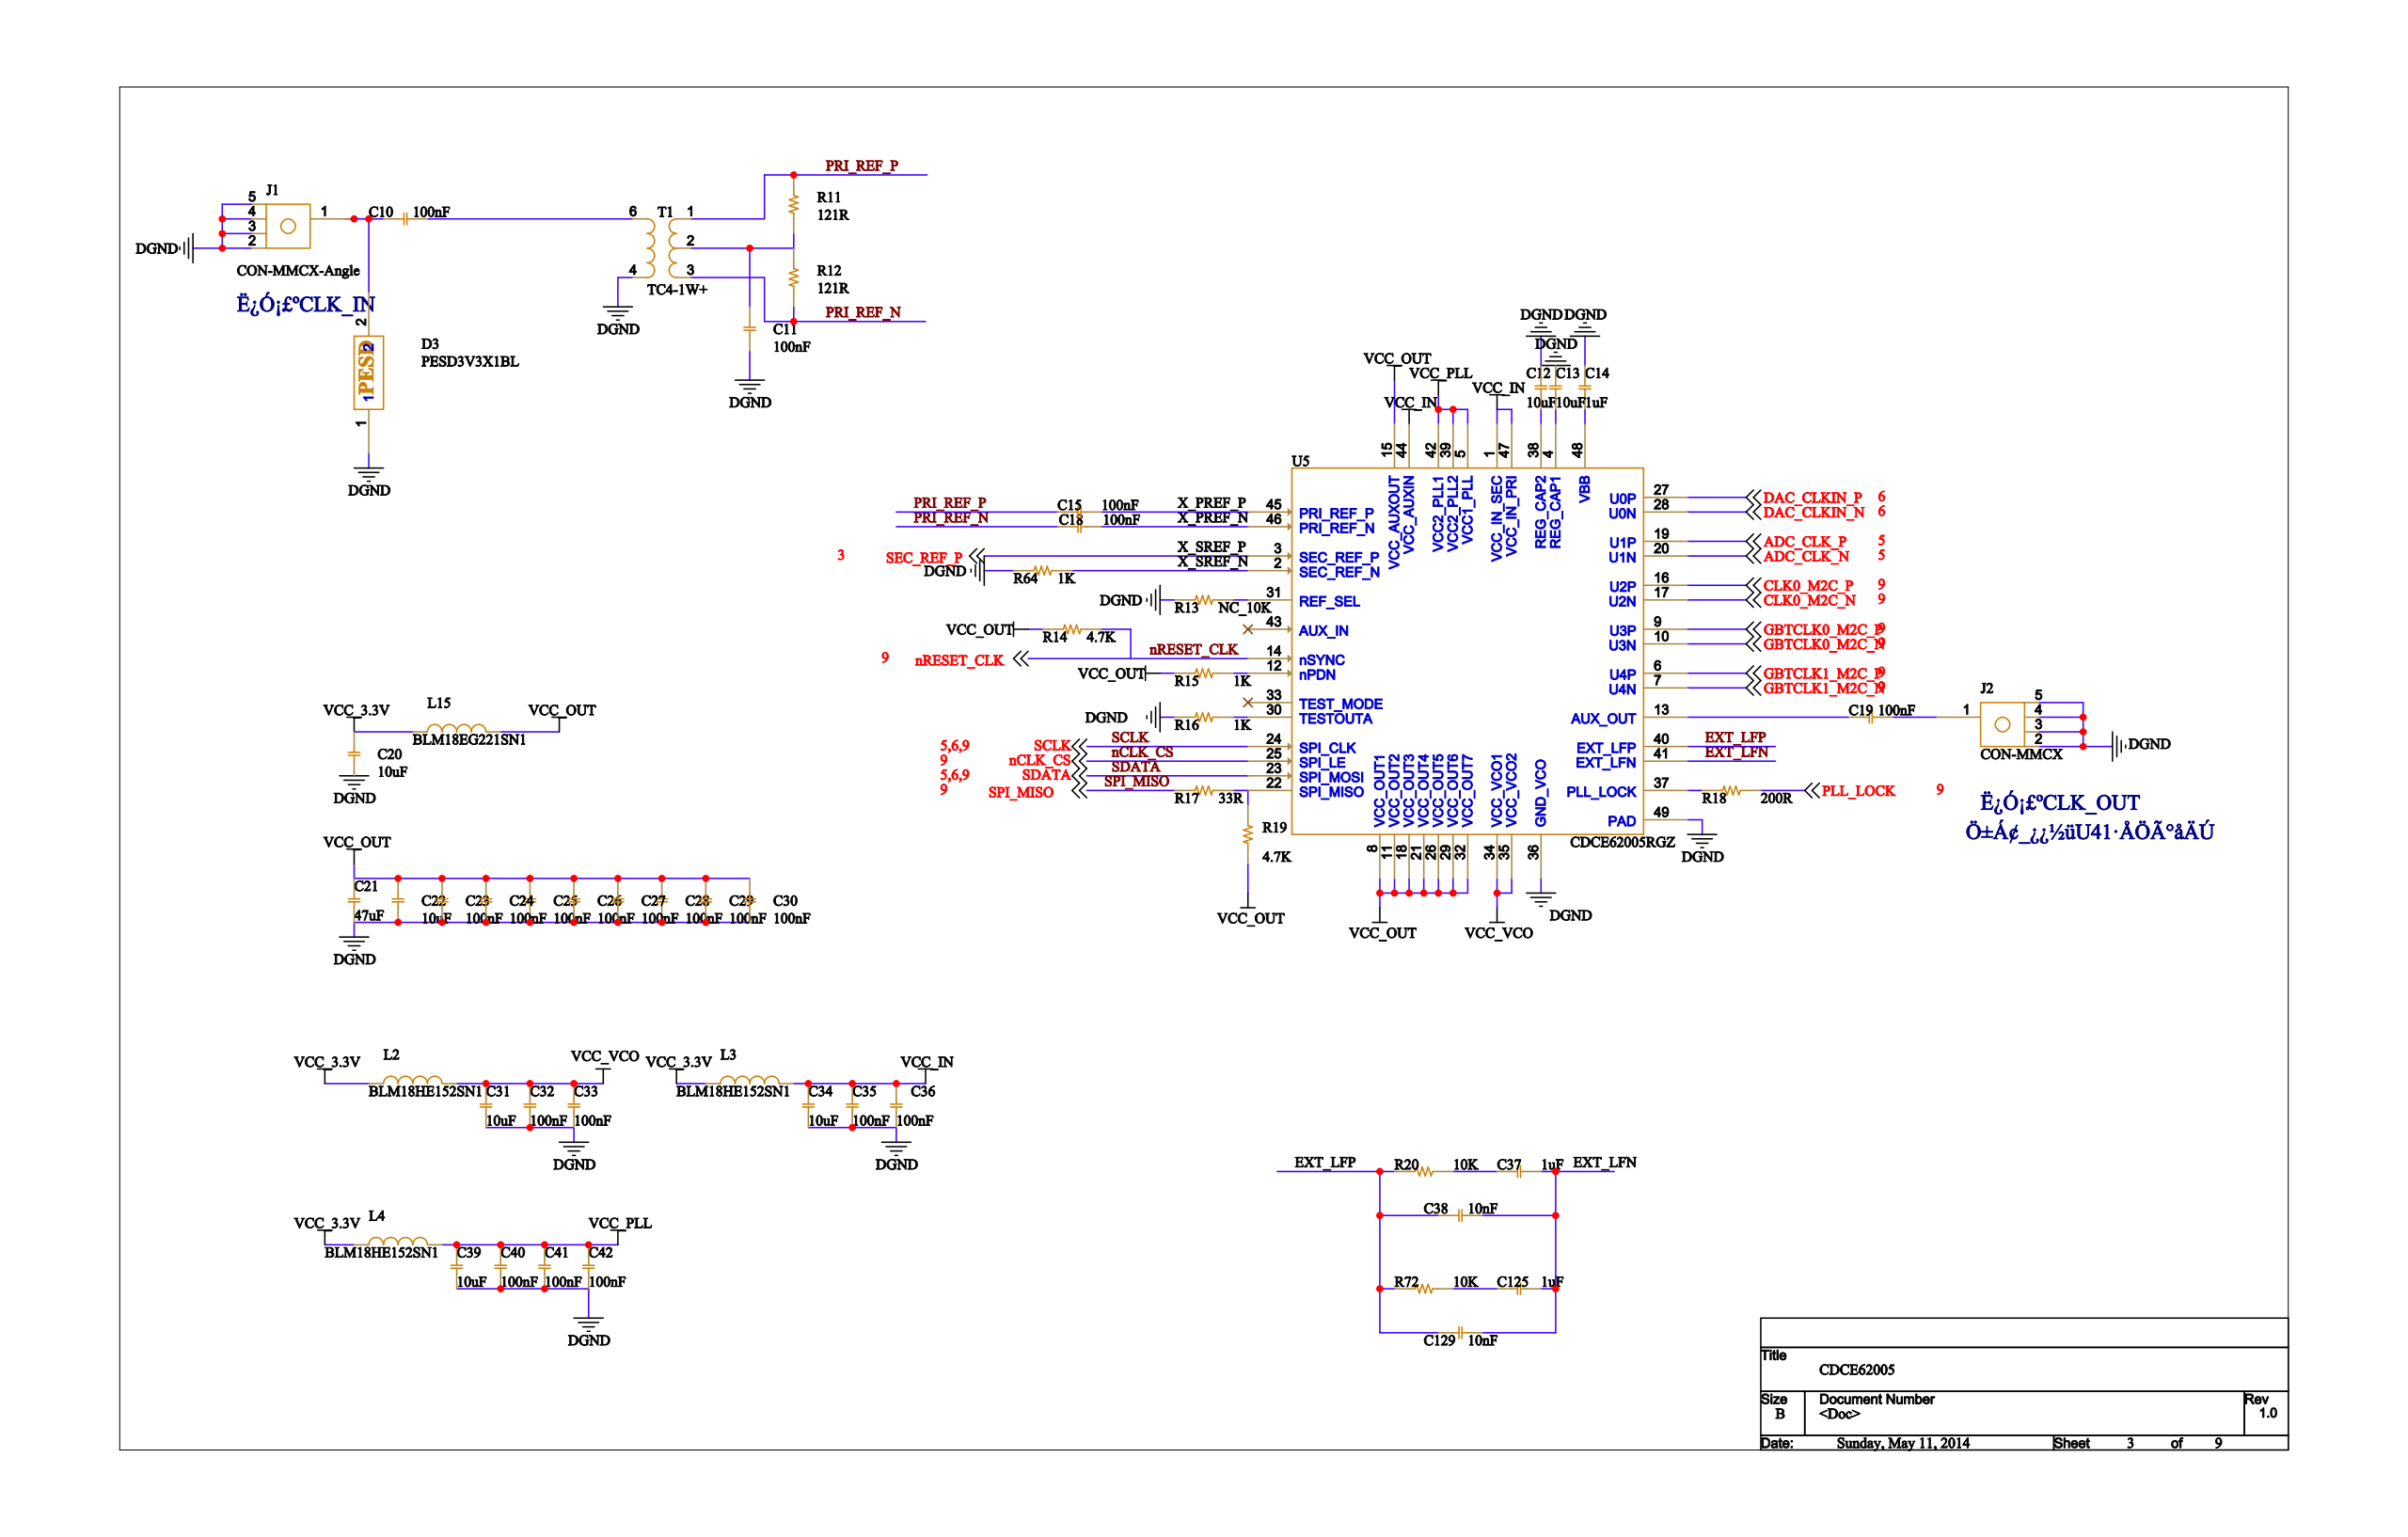Circuit board | Cadence Allegro | 233 parts | 224 nets | one sheet of the schematic
Parts on this sheet (reference | value | footprint):
C12 | 10uF | FPC-0603C
C13 | 10uF | FPC-0603C
C14 | 1uF | FPC-0402C
C15 | 100nF | FPC-0402C
C18 | 100nF | FPC-0402C
C20 | 10uF | FPC-0603C
C21 | 47uF | FPC-1206C
C22 | 10uF | FPC-0603C
C23 | 100nF | FPC-0402C
C24 | 100nF | FPC-0402C
C25 | 100nF | FPC-0402C
C26 | 100nF | FPC-0402C
C27 | 100nF | FPC-0402C
C28 | 100nF | FPC-0402C
C29 | 100nF | FPC-0402C
C30 | 100nF | FPC-0402C
C31 | 10uF | FPC-0603C
C32 | 100nF | FPC-0402C
C33 | 100nF | FPC-0402C
C34 | 10uF | FPC-0603C
C35 | 100nF | FPC-0402C
C36 | 100nF | FPC-0402C
C37 | 1uF | FPC-0603C
C38 | 10nF | FPC-0603C
C39 | 10uF | FPC-0603C
C40 | 100nF | FPC-0402C
C41 | 100nF | FPC-0402C
C42 | 100nF | FPC-0402C
C125 | 1uF | FPC-0603C
C129 | 10nF | FPC-0603C
D3 | PESD3V3X1BL | SOD882
J1 | CON-MMCX-Angle | SMA
J2 | CON-MMCX | SMA
L2 | BLM18HE152SN1 | FPC-0603L
L3 | BLM18HE152SN1 | FPC-0603L
L4 | BLM18HE152SN1 | FPC-0603L
L15 | BLM18EG221SN1 | FPC-0603L
R11 | 121R | FPC-0603R
R12 | 121R | FPC-0603R
R13 | NC_10K | FPC-0603R
R14 | 4.7K | FPC-0603R
R15 | 1K | FPC-0603R
R16 | 1K | FPC-0603R
R17 | 33R | FPC-0603R
R18 | 200R | FPC-0603R
R19 | 4.7K | FPC-0603R
R20 | 10K | FPC-0603R
R64 | 1K | FPC-0603R
R72 | 10K | FPC-0603R
T1 | TC4-1W+ | FPC-TRAN5SM-3R81X3R81
U5 | CDCE62005RGZ | FPC-QFN7X7-48-1
Nets of these parts (net: part-pin ...):
DGND: C12-2 C13-2 C14-2 C20-1 C21-2 C22-1 C23-1 C24-1 C25-1 C26-1 C27-1 C28-1 C29-1 C30-1 C31-1 C32-1 C33-1 C34-1 C35-1 C36-1 C39-1 C40-1 C41-1 C42-1 D3-1 J1-2 J1-3 J1-4 J1-5 J2-2 J2-3 J2-4 J2-5 R13-1 R16-1 R64-1 T1-4 U5-36 U5-49
N30140: D3-2 J1-1
N316817: J2-1
N75236: T1-6
VCC_3.3V: C20-2 L2-1 L3-1 L4-1 L15-1
N30096: R11-1 R12-2 T1-2
PRI_REF_P: C15-1 R11-2 T1-1
X_PREF_P: C15-2 U5-45
PRI_REF_N: C18-1 R12-1 T1-3
X_PREF_N: C18-2 U5-46
VCC_OUT: C21-1 C22-2 C23-2 C24-2 C25-2 C26-2 C27-2 C28-2 C29-2 C30-2 L15-2 R14-1 R15-1 R19-1 U5-8 U5-11 U5-15 U5-18 U5-21 U5-26 U5-29 U5-32
VCC_VCO: C31-2 C32-2 C33-2 L2-2 U5-34 U5-35
VCC_IN: C34-2 C35-2 C36-2 L3-2 U5-1 U5-44 U5-47
VCC_PLL: C39-2 C40-2 C41-2 C42-2 L4-2 U5-5 U5-39 U5-42
ADC_CLK_P: U5-19
ADC_CLK_N: U5-20
N81172: C14-1 U5-48
N27226: C12-1 U5-38
N27228: C13-1 U5-4
EXT_LFN: C37-1 C38-1 C125-1 C129-1 U5-41
N689854: C125-2 R72-2
N27340: C37-2 R20-2
EXT_LFP: C38-2 C129-2 R20-1 R72-1 U5-40
DAC_CLKIN_P: U5-27
DAC_CLKIN_N: U5-28
PLL_LOCK: R18-2
CLK0_M2C_N: U5-17
CLK0_M2C_P: U5-16
N873469: R13-2 U5-31
NRESET_CLK: R14-2 U5-14
N80647: R17-2 R19-2 U5-22
N27214: R15-2 U5-12
N873473: R16-2 U5-30
X_SREF_N: R64-2 U5-2
SPI_MISO: R17-1
SEC_REF_P: U5-3
N81195: R18-1 U5-37
SCLK: U5-24
SDATA: U5-23